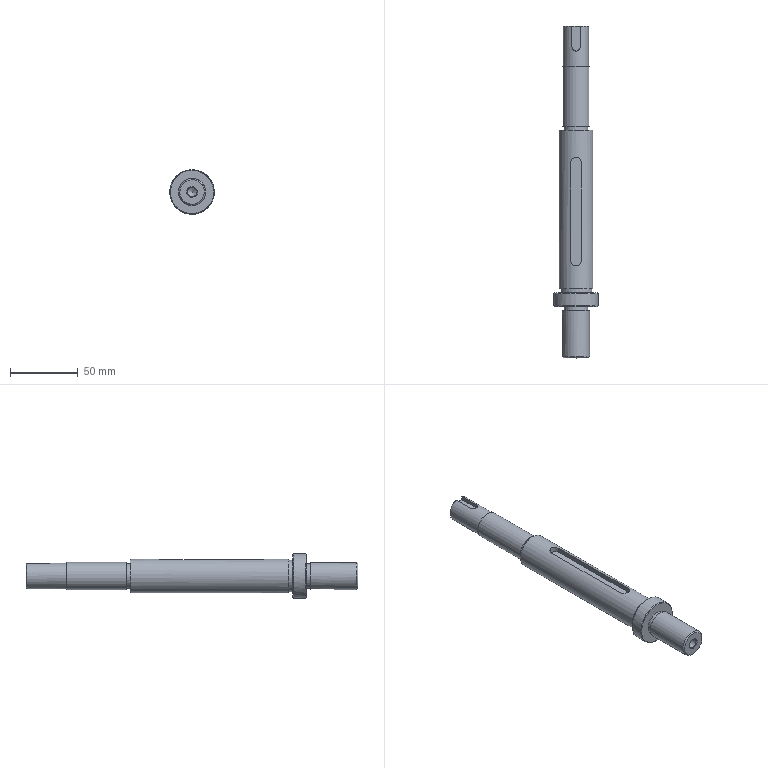Part | STEP file | YBQDJ-YB-11 | 1 solid | 33 faces | box 33 x 245 x 33 mm | volume 98573 mm3 | plane 15 | cylinder 12 | cone 6 | commonest cylinder face diameters 8.04 x2 18 x2 20 x2 6.06 x1 6.8 x1 19 x1